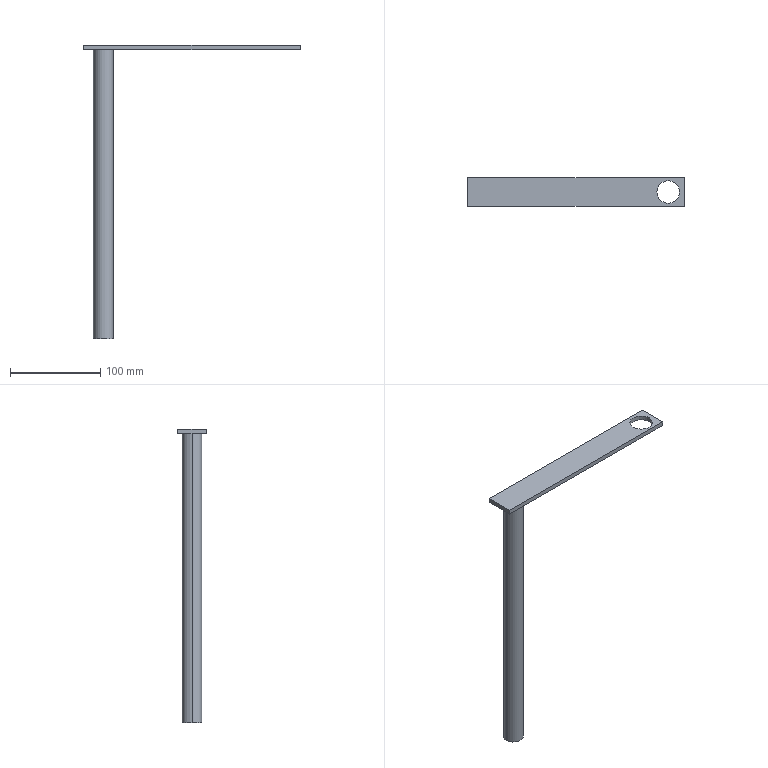Part | STEP file | 1 solid | 11 faces | box 240 x 32 x 325 mm | volume 157588 mm3 | plane 7 | cylinder 4 | commonest cylinder face diameters 22 x2 25 x2
STEP:
#1=CARTESIAN_POINT('',(0.,0.,0.));
#2=DIRECTION('',(0.,0.,1.));
#3=DIRECTION('',(1.,0.,0.));
#4=AXIS2_PLACEMENT_3D('',#1,#2,#3);
#5=CARTESIAN_POINT('',(-109.,0.,0.));
#6=VERTEX_POINT('',#5);
#7=CARTESIAN_POINT('',(-87.,0.,0.));
#8=VERTEX_POINT('',#7);
#9=CARTESIAN_POINT('',(-98.,0.,0.));
#10=DIRECTION('',(0.,0.,-1.));
#11=DIRECTION('',(-1.,0.,0.));
#12=AXIS2_PLACEMENT_3D('',#9,#10,#11);
#13=CIRCLE('',#12,11.);
#14=CARTESIAN_POINT('',(-98.,0.,-320.));
#15=DIRECTION('',(0.,0.,-1.));
#16=DIRECTION('',(-1.,0.,0.));
#17=AXIS2_PLACEMENT_3D('',#14,#15,#16);
#18=CYLINDRICAL_SURFACE('',#17,11.);
#19=CARTESIAN_POINT('',(0.,-320.));
#20=DIRECTION('',(1.,0.));
#21=VECTOR('',#20,1.);
#22=LINE('',#19,#21);
#23=(GEOMETRIC_REPRESENTATION_CONTEXT(2)PARAMETRIC_REPRESENTATION_CONTEXT()REPRESENTATION_CONTEXT('',''));
#24=DEFINITIONAL_REPRESENTATION('',(#22),#23);
#25=PCURVE('',#18,#24);
#26=CARTESIAN_POINT('',(0.,0.,0.));
#27=DIRECTION('',(0.,0.,1.));
#28=DIRECTION('',(1.,0.,0.));
#29=AXIS2_PLACEMENT_3D('',#26,#27,#28);
#30=PLANE('',#29);
#31=CARTESIAN_POINT('',(-109.,0.));
#32=CARTESIAN_POINT('',(-109.,19.053));
#33=CARTESIAN_POINT('',(-92.5,9.526));
#34=CARTESIAN_POINT('',(-76.,0.));
#35=CARTESIAN_POINT('',(-92.5,-9.526));
#36=CARTESIAN_POINT('',(-109.,-19.053));
#37=CARTESIAN_POINT('',(-109.,0.));
#38=(BOUNDED_CURVE()B_SPLINE_CURVE(2,(#31,#32,#33,#34,#35,#36,#37),.UNSPECIFIED.,.T.,.F.)B_SPLINE_CURVE_WITH_KNOTS((1,2,2,2,2,1),(-2.094,0.,2.094,4.189,6.283,8.378),.UNSPECIFIED.)CURVE()GEOMETRIC_REPRESENTATION_ITEM()RATIONAL_B_SPLINE_CURVE((1.,0.5,1.,0.5,1.,0.5,1.))REPRESENTATION_ITEM(''));
#39=(GEOMETRIC_REPRESENTATION_CONTEXT(2)PARAMETRIC_REPRESENTATION_CONTEXT()REPRESENTATION_CONTEXT('',''));
#40=DEFINITIONAL_REPRESENTATION('',(#38),#39);
#41=PCURVE('',#30,#40);
#42=SURFACE_CURVE('',#13,(#25,#41),.PCURVE_S1.);
#43=EDGE_CURVE('',#6,#8,#42,.T.);
#44=ORIENTED_EDGE('',*,*,#43,.T.);
#45=CARTESIAN_POINT('',(-87.,0.,-320.));
#46=VERTEX_POINT('',#45);
#47=CARTESIAN_POINT('',(-87.,0.,-320.));
#48=DIRECTION('',(0.,0.,-1.));
#49=VECTOR('',#48,1.);
#50=LINE('',#47,#49);
#51=CARTESIAN_POINT('',(3.142,0.));
#52=DIRECTION('',(0.,1.));
#53=VECTOR('',#52,1.);
#54=LINE('',#51,#53);
#55=(GEOMETRIC_REPRESENTATION_CONTEXT(2)PARAMETRIC_REPRESENTATION_CONTEXT()REPRESENTATION_CONTEXT('',''));
#56=DEFINITIONAL_REPRESENTATION('',(#54),#55);
#57=PCURVE('',#18,#56);
#58=CARTESIAN_POINT('',(-98.,0.,-320.));
#59=DIRECTION('',(0.,0.,-1.));
#60=DIRECTION('',(-1.,0.,0.));
#61=AXIS2_PLACEMENT_3D('',#58,#59,#60);
#62=CYLINDRICAL_SURFACE('',#61,11.);
#63=CARTESIAN_POINT('',(3.142,0.));
#64=DIRECTION('',(0.,1.));
#65=VECTOR('',#64,1.);
#66=LINE('',#63,#65);
#67=(GEOMETRIC_REPRESENTATION_CONTEXT(2)PARAMETRIC_REPRESENTATION_CONTEXT()REPRESENTATION_CONTEXT('',''));
#68=DEFINITIONAL_REPRESENTATION('',(#66),#67);
#69=PCURVE('',#62,#68);
#70=SURFACE_CURVE('',#50,(#57,#69),.PCURVE_S1.);
#71=EDGE_CURVE('',#8,#46,#70,.T.);
#72=ORIENTED_EDGE('',*,*,#71,.T.);
#73=CARTESIAN_POINT('',(-109.,0.,-320.));
#74=VERTEX_POINT('',#73);
#75=CARTESIAN_POINT('',(-98.,0.,-320.));
#76=DIRECTION('',(0.,0.,1.));
#77=DIRECTION('',(-1.,0.,0.));
#78=AXIS2_PLACEMENT_3D('',#75,#76,#77);
#79=CIRCLE('',#78,11.);
#80=CARTESIAN_POINT('',(6.283,0.));
#81=DIRECTION('',(-1.,0.));
#82=VECTOR('',#81,1.);
#83=LINE('',#80,#82);
#84=(GEOMETRIC_REPRESENTATION_CONTEXT(2)PARAMETRIC_REPRESENTATION_CONTEXT()REPRESENTATION_CONTEXT('',''));
#85=DEFINITIONAL_REPRESENTATION('',(#83),#84);
#86=PCURVE('',#18,#85);
#87=CARTESIAN_POINT('',(-98.,0.,-320.));
#88=DIRECTION('',(0.,0.,-1.));
#89=DIRECTION('',(-1.,0.,0.));
#90=AXIS2_PLACEMENT_3D('',#87,#88,#89);
#91=PLANE('',#90);
#92=CARTESIAN_POINT('',(11.,0.));
#93=CARTESIAN_POINT('',(11.,-19.053));
#94=CARTESIAN_POINT('',(-5.5,-9.526));
#95=CARTESIAN_POINT('',(-22.,0.));
#96=CARTESIAN_POINT('',(-5.5,9.526));
#97=CARTESIAN_POINT('',(11.,19.053));
#98=CARTESIAN_POINT('',(11.,0.));
#99=(BOUNDED_CURVE()B_SPLINE_CURVE(2,(#92,#93,#94,#95,#96,#97,#98),.UNSPECIFIED.,.T.,.F.)B_SPLINE_CURVE_WITH_KNOTS((1,2,2,2,2,1),(-2.094,0.,2.094,4.189,6.283,8.378),.UNSPECIFIED.)CURVE()GEOMETRIC_REPRESENTATION_ITEM()RATIONAL_B_SPLINE_CURVE((1.,0.5,1.,0.5,1.,0.5,1.))REPRESENTATION_ITEM(''));
#100=(GEOMETRIC_REPRESENTATION_CONTEXT(2)PARAMETRIC_REPRESENTATION_CONTEXT()REPRESENTATION_CONTEXT('',''));
#101=DEFINITIONAL_REPRESENTATION('',(#99),#100);
#102=PCURVE('',#91,#101);
#103=SURFACE_CURVE('',#79,(#86,#102),.PCURVE_S1.);
#104=EDGE_CURVE('',#46,#74,#103,.T.);
#105=ORIENTED_EDGE('',*,*,#104,.T.);
#106=CARTESIAN_POINT('',(-109.,0.,-320.));
#107=DIRECTION('',(0.,0.,-1.));
#108=VECTOR('',#107,1.);
#109=LINE('',#106,#108);
#110=CARTESIAN_POINT('',(0.,0.));
#111=DIRECTION('',(0.,1.));
#112=VECTOR('',#111,1.);
#113=LINE('',#110,#112);
#114=(GEOMETRIC_REPRESENTATION_CONTEXT(2)PARAMETRIC_REPRESENTATION_CONTEXT()REPRESENTATION_CONTEXT('',''));
#115=DEFINITIONAL_REPRESENTATION('',(#113),#114);
#116=PCURVE('',#18,#115);
#117=CARTESIAN_POINT('',(6.283,0.));
#118=DIRECTION('',(0.,1.));
#119=VECTOR('',#118,1.);
#120=LINE('',#117,#119);
#121=(GEOMETRIC_REPRESENTATION_CONTEXT(2)PARAMETRIC_REPRESENTATION_CONTEXT()REPRESENTATION_CONTEXT('',''));
#122=DEFINITIONAL_REPRESENTATION('',(#120),#121);
#123=PCURVE('',#62,#122);
#124=SURFACE_CURVE('',#109,(#116,#123),.PCURVE_S1.);
#125=EDGE_CURVE('',#6,#74,#124,.T.);
#126=ORIENTED_EDGE('',*,*,#125,.F.);
#127=EDGE_LOOP('',(#44,#72,#105,#126));
#128=FACE_BOUND('',#127,.T.);
#129=ADVANCED_FACE('',(#128),#18,.T.);
#130=CARTESIAN_POINT('',(89.5,0.,5.));
#131=VERTEX_POINT('',#130);
#132=CARTESIAN_POINT('',(89.5,0.,0.));
#133=VERTEX_POINT('',#132);
#134=CARTESIAN_POINT('',(89.5,0.,-18.));
#135=DIRECTION('',(0.,0.,-1.));
#136=VECTOR('',#135,1.);
#137=LINE('',#134,#136);
#138=CARTESIAN_POINT('',(102.,0.,-18.));
#139=DIRECTION('',(0.,0.,-1.));
#140=DIRECTION('',(-1.,0.,0.));
#141=AXIS2_PLACEMENT_3D('',#138,#139,#140);
#142=CYLINDRICAL_SURFACE('',#141,12.5);
#143=CARTESIAN_POINT('',(6.283,0.));
#144=DIRECTION('',(0.,1.));
#145=VECTOR('',#144,1.);
#146=LINE('',#143,#145);
#147=(GEOMETRIC_REPRESENTATION_CONTEXT(2)PARAMETRIC_REPRESENTATION_CONTEXT()REPRESENTATION_CONTEXT('',''));
#148=DEFINITIONAL_REPRESENTATION('',(#146),#147);
#149=PCURVE('',#142,#148);
#150=CARTESIAN_POINT('',(102.,0.,-18.));
#151=DIRECTION('',(0.,0.,-1.));
#152=DIRECTION('',(-1.,0.,0.));
#153=AXIS2_PLACEMENT_3D('',#150,#151,#152);
#154=CYLINDRICAL_SURFACE('',#153,12.5);
#155=CARTESIAN_POINT('',(0.,0.));
#156=DIRECTION('',(0.,1.));
#157=VECTOR('',#156,1.);
#158=LINE('',#155,#157);
#159=(GEOMETRIC_REPRESENTATION_CONTEXT(2)PARAMETRIC_REPRESENTATION_CONTEXT()REPRESENTATION_CONTEXT('',''));
#160=DEFINITIONAL_REPRESENTATION('',(#158),#159);
#161=PCURVE('',#154,#160);
#162=SURFACE_CURVE('',#137,(#149,#161),.PCURVE_S1.);
#163=EDGE_CURVE('',#131,#133,#162,.T.);
#164=ORIENTED_EDGE('',*,*,#163,.T.);
#165=CARTESIAN_POINT('',(114.5,0.,0.));
#166=VERTEX_POINT('',#165);
#167=CARTESIAN_POINT('',(102.,0.,0.));
#168=DIRECTION('',(0.,0.,-1.));
#169=DIRECTION('',(-1.,0.,0.));
#170=AXIS2_PLACEMENT_3D('',#167,#168,#169);
#171=CIRCLE('',#170,12.5);
#172=CARTESIAN_POINT('',(0.,-18.));
#173=DIRECTION('',(1.,0.));
#174=VECTOR('',#173,1.);
#175=LINE('',#172,#174);
#176=(GEOMETRIC_REPRESENTATION_CONTEXT(2)PARAMETRIC_REPRESENTATION_CONTEXT()REPRESENTATION_CONTEXT('',''));
#177=DEFINITIONAL_REPRESENTATION('',(#175),#176);
#178=PCURVE('',#142,#177);
#179=CARTESIAN_POINT('',(89.5,0.));
#180=CARTESIAN_POINT('',(89.5,21.651));
#181=CARTESIAN_POINT('',(108.25,10.825));
#182=CARTESIAN_POINT('',(127.,0.));
#183=CARTESIAN_POINT('',(108.25,-10.825));
#184=CARTESIAN_POINT('',(89.5,-21.651));
#185=CARTESIAN_POINT('',(89.5,0.));
#186=(BOUNDED_CURVE()B_SPLINE_CURVE(2,(#179,#180,#181,#182,#183,#184,#185),.UNSPECIFIED.,.T.,.F.)B_SPLINE_CURVE_WITH_KNOTS((1,2,2,2,2,1),(-2.094,0.,2.094,4.189,6.283,8.378),.UNSPECIFIED.)CURVE()GEOMETRIC_REPRESENTATION_ITEM()RATIONAL_B_SPLINE_CURVE((1.,0.5,1.,0.5,1.,0.5,1.))REPRESENTATION_ITEM(''));
#187=(GEOMETRIC_REPRESENTATION_CONTEXT(2)PARAMETRIC_REPRESENTATION_CONTEXT()REPRESENTATION_CONTEXT('',''));
#188=DEFINITIONAL_REPRESENTATION('',(#186),#187);
#189=PCURVE('',#30,#188);
#190=SURFACE_CURVE('',#171,(#178,#189),.PCURVE_S1.);
#191=EDGE_CURVE('',#166,#133,#190,.T.);
#192=ORIENTED_EDGE('',*,*,#191,.F.);
#193=CARTESIAN_POINT('',(114.5,0.,5.));
#194=VERTEX_POINT('',#193);
#195=CARTESIAN_POINT('',(114.5,0.,-18.));
#196=DIRECTION('',(0.,0.,-1.));
#197=VECTOR('',#196,1.);
#198=LINE('',#195,#197);
#199=CARTESIAN_POINT('',(3.142,0.));
#200=DIRECTION('',(0.,1.));
#201=VECTOR('',#200,1.);
#202=LINE('',#199,#201);
#203=(GEOMETRIC_REPRESENTATION_CONTEXT(2)PARAMETRIC_REPRESENTATION_CONTEXT()REPRESENTATION_CONTEXT('',''));
#204=DEFINITIONAL_REPRESENTATION('',(#202),#203);
#205=PCURVE('',#142,#204);
#206=CARTESIAN_POINT('',(3.142,0.));
#207=DIRECTION('',(0.,1.));
#208=VECTOR('',#207,1.);
#209=LINE('',#206,#208);
#210=(GEOMETRIC_REPRESENTATION_CONTEXT(2)PARAMETRIC_REPRESENTATION_CONTEXT()REPRESENTATION_CONTEXT('',''));
#211=DEFINITIONAL_REPRESENTATION('',(#209),#210);
#212=PCURVE('',#154,#211);
#213=SURFACE_CURVE('',#198,(#205,#212),.PCURVE_S1.);
#214=EDGE_CURVE('',#194,#166,#213,.T.);
#215=ORIENTED_EDGE('',*,*,#214,.F.);
#216=CARTESIAN_POINT('',(102.,0.,5.));
#217=DIRECTION('',(0.,0.,-1.));
#218=DIRECTION('',(-1.,0.,0.));
#219=AXIS2_PLACEMENT_3D('',#216,#217,#218);
#220=CIRCLE('',#219,12.5);
#221=CARTESIAN_POINT('',(0.,-23.));
#222=DIRECTION('',(1.,0.));
#223=VECTOR('',#222,1.);
#224=LINE('',#221,#223);
#225=(GEOMETRIC_REPRESENTATION_CONTEXT(2)PARAMETRIC_REPRESENTATION_CONTEXT()REPRESENTATION_CONTEXT('',''));
#226=DEFINITIONAL_REPRESENTATION('',(#224),#225);
#227=PCURVE('',#142,#226);
#228=CARTESIAN_POINT('',(0.,0.,5.));
#229=DIRECTION('',(0.,0.,1.));
#230=DIRECTION('',(1.,0.,0.));
#231=AXIS2_PLACEMENT_3D('',#228,#229,#230);
#232=PLANE('',#231);
#233=CARTESIAN_POINT('',(89.5,0.));
#234=CARTESIAN_POINT('',(89.5,21.651));
#235=CARTESIAN_POINT('',(108.25,10.825));
#236=CARTESIAN_POINT('',(127.,0.));
#237=CARTESIAN_POINT('',(108.25,-10.825));
#238=CARTESIAN_POINT('',(89.5,-21.651));
#239=CARTESIAN_POINT('',(89.5,0.));
#240=(BOUNDED_CURVE()B_SPLINE_CURVE(2,(#233,#234,#235,#236,#237,#238,#239),.UNSPECIFIED.,.T.,.F.)B_SPLINE_CURVE_WITH_KNOTS((1,2,2,2,2,1),(-2.094,0.,2.094,4.189,6.283,8.378),.UNSPECIFIED.)CURVE()GEOMETRIC_REPRESENTATION_ITEM()RATIONAL_B_SPLINE_CURVE((1.,0.5,1.,0.5,1.,0.5,1.))REPRESENTATION_ITEM(''));
#241=(GEOMETRIC_REPRESENTATION_CONTEXT(2)PARAMETRIC_REPRESENTATION_CONTEXT()REPRESENTATION_CONTEXT('',''));
#242=DEFINITIONAL_REPRESENTATION('',(#240),#241);
#243=PCURVE('',#232,#242);
#244=SURFACE_CURVE('',#220,(#227,#243),.PCURVE_S1.);
#245=EDGE_CURVE('',#194,#131,#244,.T.);
#246=ORIENTED_EDGE('',*,*,#245,.T.);
#247=EDGE_LOOP('',(#164,#192,#215,#246));
#248=FACE_BOUND('',#247,.F.);
#249=ADVANCED_FACE('',(#248),#142,.F.);
#250=ORIENTED_EDGE('',*,*,#71,.F.);
#251=CARTESIAN_POINT('',(-98.,0.,0.));
#252=DIRECTION('',(0.,0.,-1.));
#253=DIRECTION('',(-1.,0.,0.));
#254=AXIS2_PLACEMENT_3D('',#251,#252,#253);
#255=CIRCLE('',#254,11.);
#256=CARTESIAN_POINT('',(0.,-320.));
#257=DIRECTION('',(1.,0.));
#258=VECTOR('',#257,1.);
#259=LINE('',#256,#258);
#260=(GEOMETRIC_REPRESENTATION_CONTEXT(2)PARAMETRIC_REPRESENTATION_CONTEXT()REPRESENTATION_CONTEXT('',''));
#261=DEFINITIONAL_REPRESENTATION('',(#259),#260);
#262=PCURVE('',#62,#261);
#263=CARTESIAN_POINT('',(-109.,0.));
#264=CARTESIAN_POINT('',(-109.,19.053));
#265=CARTESIAN_POINT('',(-92.5,9.526));
#266=CARTESIAN_POINT('',(-76.,0.));
#267=CARTESIAN_POINT('',(-92.5,-9.526));
#268=CARTESIAN_POINT('',(-109.,-19.053));
#269=CARTESIAN_POINT('',(-109.,0.));
#270=(BOUNDED_CURVE()B_SPLINE_CURVE(2,(#263,#264,#265,#266,#267,#268,#269),.UNSPECIFIED.,.T.,.F.)B_SPLINE_CURVE_WITH_KNOTS((1,2,2,2,2,1),(-2.094,0.,2.094,4.189,6.283,8.378),.UNSPECIFIED.)CURVE()GEOMETRIC_REPRESENTATION_ITEM()RATIONAL_B_SPLINE_CURVE((1.,0.5,1.,0.5,1.,0.5,1.))REPRESENTATION_ITEM(''));
#271=(GEOMETRIC_REPRESENTATION_CONTEXT(2)PARAMETRIC_REPRESENTATION_CONTEXT()REPRESENTATION_CONTEXT('',''));
#272=DEFINITIONAL_REPRESENTATION('',(#270),#271);
#273=PCURVE('',#30,#272);
#274=SURFACE_CURVE('',#255,(#262,#273),.PCURVE_S1.);
#275=EDGE_CURVE('',#8,#6,#274,.T.);
#276=ORIENTED_EDGE('',*,*,#275,.T.);
#277=ORIENTED_EDGE('',*,*,#125,.T.);
#278=CARTESIAN_POINT('',(-98.,0.,-320.));
#279=DIRECTION('',(0.,0.,1.));
#280=DIRECTION('',(-1.,0.,0.));
#281=AXIS2_PLACEMENT_3D('',#278,#279,#280);
#282=CIRCLE('',#281,11.);
#283=CARTESIAN_POINT('',(6.283,0.));
#284=DIRECTION('',(-1.,0.));
#285=VECTOR('',#284,1.);
#286=LINE('',#283,#285);
#287=(GEOMETRIC_REPRESENTATION_CONTEXT(2)PARAMETRIC_REPRESENTATION_CONTEXT()REPRESENTATION_CONTEXT('',''));
#288=DEFINITIONAL_REPRESENTATION('',(#286),#287);
#289=PCURVE('',#62,#288);
#290=CARTESIAN_POINT('',(11.,0.));
#291=CARTESIAN_POINT('',(11.,-19.053));
#292=CARTESIAN_POINT('',(-5.5,-9.526));
#293=CARTESIAN_POINT('',(-22.,0.));
#294=CARTESIAN_POINT('',(-5.5,9.526));
#295=CARTESIAN_POINT('',(11.,19.053));
#296=CARTESIAN_POINT('',(11.,0.));
#297=(BOUNDED_CURVE()B_SPLINE_CURVE(2,(#290,#291,#292,#293,#294,#295,#296),.UNSPECIFIED.,.T.,.F.)B_SPLINE_CURVE_WITH_KNOTS((1,2,2,2,2,1),(-2.094,0.,2.094,4.189,6.283,8.378),.UNSPECIFIED.)CURVE()GEOMETRIC_REPRESENTATION_ITEM()RATIONAL_B_SPLINE_CURVE((1.,0.5,1.,0.5,1.,0.5,1.))REPRESENTATION_ITEM(''));
#298=(GEOMETRIC_REPRESENTATION_CONTEXT(2)PARAMETRIC_REPRESENTATION_CONTEXT()REPRESENTATION_CONTEXT('',''));
#299=DEFINITIONAL_REPRESENTATION('',(#297),#298);
#300=PCURVE('',#91,#299);
#301=SURFACE_CURVE('',#282,(#289,#300),.PCURVE_S1.);
#302=EDGE_CURVE('',#74,#46,#301,.T.);
#303=ORIENTED_EDGE('',*,*,#302,.T.);
#304=EDGE_LOOP('',(#250,#276,#277,#303));
#305=FACE_BOUND('',#304,.T.);
#306=ADVANCED_FACE('',(#305),#62,.T.);
#307=CARTESIAN_POINT('',(102.,0.,0.));
#308=DIRECTION('',(0.,0.,-1.));
#309=DIRECTION('',(-1.,0.,0.));
#310=AXIS2_PLACEMENT_3D('',#307,#308,#309);
#311=CIRCLE('',#310,12.5);
#312=CARTESIAN_POINT('',(89.5,0.));
#313=CARTESIAN_POINT('',(89.5,21.651));
#314=CARTESIAN_POINT('',(108.25,10.825));
#315=CARTESIAN_POINT('',(127.,0.));
#316=CARTESIAN_POINT('',(108.25,-10.825));
#317=CARTESIAN_POINT('',(89.5,-21.651));
#318=CARTESIAN_POINT('',(89.5,0.));
#319=(BOUNDED_CURVE()B_SPLINE_CURVE(2,(#312,#313,#314,#315,#316,#317,#318),.UNSPECIFIED.,.T.,.F.)B_SPLINE_CURVE_WITH_KNOTS((1,2,2,2,2,1),(-2.094,0.,2.094,4.189,6.283,8.378),.UNSPECIFIED.)CURVE()GEOMETRIC_REPRESENTATION_ITEM()RATIONAL_B_SPLINE_CURVE((1.,0.5,1.,0.5,1.,0.5,1.))REPRESENTATION_ITEM(''));
#320=(GEOMETRIC_REPRESENTATION_CONTEXT(2)PARAMETRIC_REPRESENTATION_CONTEXT()REPRESENTATION_CONTEXT('',''));
#321=DEFINITIONAL_REPRESENTATION('',(#319),#320);
#322=PCURVE('',#30,#321);
#323=CARTESIAN_POINT('',(0.,-18.));
#324=DIRECTION('',(1.,0.));
#325=VECTOR('',#324,1.);
#326=LINE('',#323,#325);
#327=(GEOMETRIC_REPRESENTATION_CONTEXT(2)PARAMETRIC_REPRESENTATION_CONTEXT()REPRESENTATION_CONTEXT('',''));
#328=DEFINITIONAL_REPRESENTATION('',(#326),#327);
#329=PCURVE('',#154,#328);
#330=SURFACE_CURVE('',#311,(#322,#329),.PCURVE_S1.);
#331=EDGE_CURVE('',#133,#166,#330,.T.);
#332=ORIENTED_EDGE('',*,*,#331,.F.);
#333=ORIENTED_EDGE('',*,*,#191,.F.);
#334=EDGE_LOOP('',(#332,#333));
#335=FACE_BOUND('',#334,.T.);
#336=ORIENTED_EDGE('',*,*,#43,.F.);
#337=ORIENTED_EDGE('',*,*,#275,.F.);
#338=EDGE_LOOP('',(#336,#337));
#339=FACE_BOUND('',#338,.T.);
#340=CARTESIAN_POINT('',(-120.,-16.,0.));
#341=VERTEX_POINT('',#340);
#342=CARTESIAN_POINT('',(120.,-16.,0.));
#343=VERTEX_POINT('',#342);
#344=CARTESIAN_POINT('',(0.,-16.,0.));
#345=DIRECTION('',(1.,0.,0.));
#346=VECTOR('',#345,1.);
#347=LINE('',#344,#346);
#348=CARTESIAN_POINT('',(0.,-16.));
#349=DIRECTION('',(1.,0.));
#350=VECTOR('',#349,1.);
#351=LINE('',#348,#350);
#352=(GEOMETRIC_REPRESENTATION_CONTEXT(2)PARAMETRIC_REPRESENTATION_CONTEXT()REPRESENTATION_CONTEXT('',''));
#353=DEFINITIONAL_REPRESENTATION('',(#351),#352);
#354=PCURVE('',#30,#353);
#355=CARTESIAN_POINT('',(-120.,-16.,5.));
#356=DIRECTION('',(0.,1.,0.));
#357=DIRECTION('',(0.,0.,1.));
#358=AXIS2_PLACEMENT_3D('',#355,#356,#357);
#359=PLANE('',#358);
#360=CARTESIAN_POINT('',(-5.,120.));
#361=DIRECTION('',(0.,1.));
#362=VECTOR('',#361,1.);
#363=LINE('',#360,#362);
#364=(GEOMETRIC_REPRESENTATION_CONTEXT(2)PARAMETRIC_REPRESENTATION_CONTEXT()REPRESENTATION_CONTEXT('',''));
#365=DEFINITIONAL_REPRESENTATION('',(#363),#364);
#366=PCURVE('',#359,#365);
#367=SURFACE_CURVE('',#347,(#354,#366),.PCURVE_S1.);
#368=EDGE_CURVE('',#341,#343,#367,.T.);
#369=ORIENTED_EDGE('',*,*,#368,.F.);
#370=CARTESIAN_POINT('',(-120.,16.,0.));
#371=VERTEX_POINT('',#370);
#372=CARTESIAN_POINT('',(-120.,0.,0.));
#373=DIRECTION('',(0.,-1.,0.));
#374=VECTOR('',#373,1.);
#375=LINE('',#372,#374);
#376=CARTESIAN_POINT('',(-120.,0.));
#377=DIRECTION('',(0.,-1.));
#378=VECTOR('',#377,1.);
#379=LINE('',#376,#378);
#380=(GEOMETRIC_REPRESENTATION_CONTEXT(2)PARAMETRIC_REPRESENTATION_CONTEXT()REPRESENTATION_CONTEXT('',''));
#381=DEFINITIONAL_REPRESENTATION('',(#379),#380);
#382=PCURVE('',#30,#381);
#383=CARTESIAN_POINT('',(-120.,16.,5.));
#384=DIRECTION('',(1.,0.,0.));
#385=DIRECTION('',(0.,0.,-1.));
#386=AXIS2_PLACEMENT_3D('',#383,#384,#385);
#387=PLANE('',#386);
#388=CARTESIAN_POINT('',(5.,-16.));
#389=DIRECTION('',(0.,-1.));
#390=VECTOR('',#389,1.);
#391=LINE('',#388,#390);
#392=(GEOMETRIC_REPRESENTATION_CONTEXT(2)PARAMETRIC_REPRESENTATION_CONTEXT()REPRESENTATION_CONTEXT('',''));
#393=DEFINITIONAL_REPRESENTATION('',(#391),#392);
#394=PCURVE('',#387,#393);
#395=SURFACE_CURVE('',#375,(#382,#394),.PCURVE_S1.);
#396=EDGE_CURVE('',#371,#341,#395,.T.);
#397=ORIENTED_EDGE('',*,*,#396,.F.);
#398=CARTESIAN_POINT('',(120.,16.,0.));
#399=VERTEX_POINT('',#398);
#400=CARTESIAN_POINT('',(0.,16.,0.));
#401=DIRECTION('',(-1.,0.,0.));
#402=VECTOR('',#401,1.);
#403=LINE('',#400,#402);
#404=CARTESIAN_POINT('',(0.,16.));
#405=DIRECTION('',(-1.,0.));
#406=VECTOR('',#405,1.);
#407=LINE('',#404,#406);
#408=(GEOMETRIC_REPRESENTATION_CONTEXT(2)PARAMETRIC_REPRESENTATION_CONTEXT()REPRESENTATION_CONTEXT('',''));
#409=DEFINITIONAL_REPRESENTATION('',(#407),#408);
#410=PCURVE('',#30,#409);
#411=CARTESIAN_POINT('',(-120.,16.,5.));
#412=DIRECTION('',(0.,-1.,0.));
#413=DIRECTION('',(0.,0.,-1.));
#414=AXIS2_PLACEMENT_3D('',#411,#412,#413);
#415=PLANE('',#414);
#416=CARTESIAN_POINT('',(5.,120.));
#417=DIRECTION('',(0.,-1.));
#418=VECTOR('',#417,1.);
#419=LINE('',#416,#418);
#420=(GEOMETRIC_REPRESENTATION_CONTEXT(2)PARAMETRIC_REPRESENTATION_CONTEXT()REPRESENTATION_CONTEXT('',''));
#421=DEFINITIONAL_REPRESENTATION('',(#419),#420);
#422=PCURVE('',#415,#421);
#423=SURFACE_CURVE('',#403,(#410,#422),.PCURVE_S1.);
#424=EDGE_CURVE('',#399,#371,#423,.T.);
#425=ORIENTED_EDGE('',*,*,#424,.F.);
#426=CARTESIAN_POINT('',(120.,0.,0.));
#427=DIRECTION('',(0.,1.,0.));
#428=VECTOR('',#427,1.);
#429=LINE('',#426,#428);
#430=CARTESIAN_POINT('',(120.,0.));
#431=DIRECTION('',(0.,1.));
#432=VECTOR('',#431,1.);
#433=LINE('',#430,#432);
#434=(GEOMETRIC_REPRESENTATION_CONTEXT(2)PARAMETRIC_REPRESENTATION_CONTEXT()REPRESENTATION_CONTEXT('',''));
#435=DEFINITIONAL_REPRESENTATION('',(#433),#434);
#436=PCURVE('',#30,#435);
#437=CARTESIAN_POINT('',(120.,16.,5.));
#438=DIRECTION('',(-1.,0.,0.));
#439=DIRECTION('',(0.,0.,1.));
#440=AXIS2_PLACEMENT_3D('',#437,#438,#439);
#441=PLANE('',#440);
#442=CARTESIAN_POINT('',(-5.,-16.));
#443=DIRECTION('',(0.,1.));
#444=VECTOR('',#443,1.);
#445=LINE('',#442,#444);
#446=(GEOMETRIC_REPRESENTATION_CONTEXT(2)PARAMETRIC_REPRESENTATION_CONTEXT()REPRESENTATION_CONTEXT('',''));
#447=DEFINITIONAL_REPRESENTATION('',(#445),#446);
#448=PCURVE('',#441,#447);
#449=SURFACE_CURVE('',#429,(#436,#448),.PCURVE_S1.);
#450=EDGE_CURVE('',#343,#399,#449,.T.);
#451=ORIENTED_EDGE('',*,*,#450,.F.);
#452=EDGE_LOOP('',(#369,#397,#425,#451));
#453=FACE_BOUND('',#452,.T.);
#454=ADVANCED_FACE('',(#335,#339,#453),#30,.F.);
#455=ORIENTED_EDGE('',*,*,#302,.F.);
#456=ORIENTED_EDGE('',*,*,#104,.F.);
#457=EDGE_LOOP('',(#455,#456));
#458=FACE_BOUND('',#457,.T.);
#459=ADVANCED_FACE('',(#458),#91,.T.);
#460=ORIENTED_EDGE('',*,*,#331,.F.);
#461=ORIENTED_EDGE('',*,*,#163,.F.);
#462=CARTESIAN_POINT('',(102.,0.,5.));
#463=DIRECTION('',(0.,0.,-1.));
#464=DIRECTION('',(-1.,0.,0.));
#465=AXIS2_PLACEMENT_3D('',#462,#463,#464);
#466=CIRCLE('',#465,12.5);
#467=CARTESIAN_POINT('',(0.,-23.));
#468=DIRECTION('',(1.,0.));
#469=VECTOR('',#468,1.);
#470=LINE('',#467,#469);
#471=(GEOMETRIC_REPRESENTATION_CONTEXT(2)PARAMETRIC_REPRESENTATION_CONTEXT()REPRESENTATION_CONTEXT('',''));
#472=DEFINITIONAL_REPRESENTATION('',(#470),#471);
#473=PCURVE('',#154,#472);
#474=CARTESIAN_POINT('',(89.5,0.));
#475=CARTESIAN_POINT('',(89.5,21.651));
#476=CARTESIAN_POINT('',(108.25,10.825));
#477=CARTESIAN_POINT('',(127.,0.));
#478=CARTESIAN_POINT('',(108.25,-10.825));
#479=CARTESIAN_POINT('',(89.5,-21.651));
#480=CARTESIAN_POINT('',(89.5,0.));
#481=(BOUNDED_CURVE()B_SPLINE_CURVE(2,(#474,#475,#476,#477,#478,#479,#480),.UNSPECIFIED.,.T.,.F.)B_SPLINE_CURVE_WITH_KNOTS((1,2,2,2,2,1),(-2.094,0.,2.094,4.189,6.283,8.378),.UNSPECIFIED.)CURVE()GEOMETRIC_REPRESENTATION_ITEM()RATIONAL_B_SPLINE_CURVE((1.,0.5,1.,0.5,1.,0.5,1.))REPRESENTATION_ITEM(''));
#482=(GEOMETRIC_REPRESENTATION_CONTEXT(2)PARAMETRIC_REPRESENTATION_CONTEXT()REPRESENTATION_CONTEXT('',''));
#483=DEFINITIONAL_REPRESENTATION('',(#481),#482);
#484=PCURVE('',#232,#483);
#485=SURFACE_CURVE('',#466,(#473,#484),.PCURVE_S1.);
#486=EDGE_CURVE('',#131,#194,#485,.T.);
#487=ORIENTED_EDGE('',*,*,#486,.T.);
#488=ORIENTED_EDGE('',*,*,#214,.T.);
#489=EDGE_LOOP('',(#460,#461,#487,#488));
#490=FACE_BOUND('',#489,.F.);
#491=ADVANCED_FACE('',(#490),#154,.F.);
#492=CARTESIAN_POINT('',(120.,16.,5.));
#493=VERTEX_POINT('',#492);
#494=CARTESIAN_POINT('',(120.,16.,5.));
#495=DIRECTION('',(0.,0.,-1.));
#496=VECTOR('',#495,1.);
#497=LINE('',#494,#496);
#498=CARTESIAN_POINT('',(0.,0.));
#499=DIRECTION('',(-1.,0.));
#500=VECTOR('',#499,1.);
#501=LINE('',#498,#500);
#502=(GEOMETRIC_REPRESENTATION_CONTEXT(2)PARAMETRIC_REPRESENTATION_CONTEXT()REPRESENTATION_CONTEXT('',''));
#503=DEFINITIONAL_REPRESENTATION('',(#501),#502);
#504=PCURVE('',#441,#503);
#505=CARTESIAN_POINT('',(0.,240.));
#506=DIRECTION('',(1.,0.));
#507=VECTOR('',#506,1.);
#508=LINE('',#505,#507);
#509=(GEOMETRIC_REPRESENTATION_CONTEXT(2)PARAMETRIC_REPRESENTATION_CONTEXT()REPRESENTATION_CONTEXT('',''));
#510=DEFINITIONAL_REPRESENTATION('',(#508),#509);
#511=PCURVE('',#415,#510);
#512=SURFACE_CURVE('',#497,(#504,#511),.PCURVE_S1.);
#513=EDGE_CURVE('',#493,#399,#512,.T.);
#514=ORIENTED_EDGE('',*,*,#513,.F.);
#515=CARTESIAN_POINT('',(120.,-16.,5.));
#516=VERTEX_POINT('',#515);
#517=CARTESIAN_POINT('',(120.,16.,5.));
#518=DIRECTION('',(0.,1.,0.));
#519=VECTOR('',#518,1.);
#520=LINE('',#517,#519);
#521=CARTESIAN_POINT('',(0.,0.));
#522=DIRECTION('',(0.,1.));
#523=VECTOR('',#522,1.);
#524=LINE('',#521,#523);
#525=(GEOMETRIC_REPRESENTATION_CONTEXT(2)PARAMETRIC_REPRESENTATION_CONTEXT()REPRESENTATION_CONTEXT('',''));
#526=DEFINITIONAL_REPRESENTATION('',(#524),#525);
#527=PCURVE('',#441,#526);
#528=CARTESIAN_POINT('',(120.,16.));
#529=DIRECTION('',(0.,1.));
#530=VECTOR('',#529,1.);
#531=LINE('',#528,#530);
#532=(GEOMETRIC_REPRESENTATION_CONTEXT(2)PARAMETRIC_REPRESENTATION_CONTEXT()REPRESENTATION_CONTEXT('',''));
#533=DEFINITIONAL_REPRESENTATION('',(#531),#532);
#534=PCURVE('',#232,#533);
#535=SURFACE_CURVE('',#520,(#527,#534),.PCURVE_S1.);
#536=EDGE_CURVE('',#516,#493,#535,.T.);
#537=ORIENTED_EDGE('',*,*,#536,.F.);
#538=CARTESIAN_POINT('',(120.,-16.,5.));
#539=DIRECTION('',(0.,0.,1.));
#540=VECTOR('',#539,1.);
#541=LINE('',#538,#540);
#542=CARTESIAN_POINT('',(0.,-32.));
#543=DIRECTION('',(1.,0.));
#544=VECTOR('',#543,1.);
#545=LINE('',#542,#544);
#546=(GEOMETRIC_REPRESENTATION_CONTEXT(2)PARAMETRIC_REPRESENTATION_CONTEXT()REPRESENTATION_CONTEXT('',''));
#547=DEFINITIONAL_REPRESENTATION('',(#545),#546);
#548=PCURVE('',#441,#547);
#549=CARTESIAN_POINT('',(0.,240.));
#550=DIRECTION('',(1.,0.));
#551=VECTOR('',#550,1.);
#552=LINE('',#549,#551);
#553=(GEOMETRIC_REPRESENTATION_CONTEXT(2)PARAMETRIC_REPRESENTATION_CONTEXT()REPRESENTATION_CONTEXT('',''));
#554=DEFINITIONAL_REPRESENTATION('',(#552),#553);
#555=PCURVE('',#359,#554);
#556=SURFACE_CURVE('',#541,(#548,#555),.PCURVE_S1.);
#557=EDGE_CURVE('',#343,#516,#556,.T.);
#558=ORIENTED_EDGE('',*,*,#557,.F.);
#559=ORIENTED_EDGE('',*,*,#450,.T.);
#560=EDGE_LOOP('',(#514,#537,#558,#559));
#561=FACE_BOUND('',#560,.T.);
#562=ADVANCED_FACE('',(#561),#441,.F.);
#563=ORIENTED_EDGE('',*,*,#557,.T.);
#564=CARTESIAN_POINT('',(-120.,-16.,5.));
#565=VERTEX_POINT('',#564);
#566=CARTESIAN_POINT('',(-120.,-16.,5.));
#567=DIRECTION('',(1.,0.,0.));
#568=VECTOR('',#567,1.);
#569=LINE('',#566,#568);
#570=CARTESIAN_POINT('',(0.,0.));
#571=DIRECTION('',(0.,1.));
#572=VECTOR('',#571,1.);
#573=LINE('',#570,#572);
#574=(GEOMETRIC_REPRESENTATION_CONTEXT(2)PARAMETRIC_REPRESENTATION_CONTEXT()REPRESENTATION_CONTEXT('',''));
#575=DEFINITIONAL_REPRESENTATION('',(#573),#574);
#576=PCURVE('',#359,#575);
#577=CARTESIAN_POINT('',(-120.,-16.));
#578=DIRECTION('',(1.,0.));
#579=VECTOR('',#578,1.);
#580=LINE('',#577,#579);
#581=(GEOMETRIC_REPRESENTATION_CONTEXT(2)PARAMETRIC_REPRESENTATION_CONTEXT()REPRESENTATION_CONTEXT('',''));
#582=DEFINITIONAL_REPRESENTATION('',(#580),#581);
#583=PCURVE('',#232,#582);
#584=SURFACE_CURVE('',#569,(#576,#583),.PCURVE_S1.);
#585=EDGE_CURVE('',#565,#516,#584,.T.);
#586=ORIENTED_EDGE('',*,*,#585,.F.);
#587=CARTESIAN_POINT('',(-120.,-16.,5.));
#588=DIRECTION('',(0.,0.,1.));
#589=VECTOR('',#588,1.);
#590=LINE('',#587,#589);
#591=CARTESIAN_POINT('',(0.,0.));
#592=DIRECTION('',(1.,0.));
#593=VECTOR('',#592,1.);
#594=LINE('',#591,#593);
#595=(GEOMETRIC_REPRESENTATION_CONTEXT(2)PARAMETRIC_REPRESENTATION_CONTEXT()REPRESENTATION_CONTEXT('',''));
#596=DEFINITIONAL_REPRESENTATION('',(#594),#595);
#597=PCURVE('',#359,#596);
#598=CARTESIAN_POINT('',(0.,-32.));
#599=DIRECTION('',(-1.,0.));
#600=VECTOR('',#599,1.);
#601=LINE('',#598,#600);
#602=(GEOMETRIC_REPRESENTATION_CONTEXT(2)PARAMETRIC_REPRESENTATION_CONTEXT()REPRESENTATION_CONTEXT('',''));
#603=DEFINITIONAL_REPRESENTATION('',(#601),#602);
#604=PCURVE('',#387,#603);
#605=SURFACE_CURVE('',#590,(#597,#604),.PCURVE_S1.);
#606=EDGE_CURVE('',#341,#565,#605,.T.);
#607=ORIENTED_EDGE('',*,*,#606,.F.);
#608=ORIENTED_EDGE('',*,*,#368,.T.);
#609=EDGE_LOOP('',(#563,#586,#607,#608));
#610=FACE_BOUND('',#609,.T.);
#611=ADVANCED_FACE('',(#610),#359,.F.);
#612=ORIENTED_EDGE('',*,*,#606,.T.);
#613=CARTESIAN_POINT('',(-120.,16.,5.));
#614=VERTEX_POINT('',#613);
#615=CARTESIAN_POINT('',(-120.,16.,5.));
#616=DIRECTION('',(0.,-1.,0.));
#617=VECTOR('',#616,1.);
#618=LINE('',#615,#617);
#619=CARTESIAN_POINT('',(0.,0.));
#620=DIRECTION('',(0.,-1.));
#621=VECTOR('',#620,1.);
#622=LINE('',#619,#621);
#623=(GEOMETRIC_REPRESENTATION_CONTEXT(2)PARAMETRIC_REPRESENTATION_CONTEXT()REPRESENTATION_CONTEXT('',''));
#624=DEFINITIONAL_REPRESENTATION('',(#622),#623);
#625=PCURVE('',#387,#624);
#626=CARTESIAN_POINT('',(-120.,16.));
#627=DIRECTION('',(0.,-1.));
#628=VECTOR('',#627,1.);
#629=LINE('',#626,#628);
#630=(GEOMETRIC_REPRESENTATION_CONTEXT(2)PARAMETRIC_REPRESENTATION_CONTEXT()REPRESENTATION_CONTEXT('',''));
#631=DEFINITIONAL_REPRESENTATION('',(#629),#630);
#632=PCURVE('',#232,#631);
#633=SURFACE_CURVE('',#618,(#625,#632),.PCURVE_S1.);
#634=EDGE_CURVE('',#614,#565,#633,.T.);
#635=ORIENTED_EDGE('',*,*,#634,.F.);
#636=CARTESIAN_POINT('',(-120.,16.,5.));
#637=DIRECTION('',(0.,0.,1.));
#638=VECTOR('',#637,1.);
#639=LINE('',#636,#638);
#640=CARTESIAN_POINT('',(0.,0.));
#641=DIRECTION('',(-1.,0.));
#642=VECTOR('',#641,1.);
#643=LINE('',#640,#642);
#644=(GEOMETRIC_REPRESENTATION_CONTEXT(2)PARAMETRIC_REPRESENTATION_CONTEXT()REPRESENTATION_CONTEXT('',''));
#645=DEFINITIONAL_REPRESENTATION('',(#643),#644);
#646=PCURVE('',#387,#645);
#647=CARTESIAN_POINT('',(0.,0.));
#648=DIRECTION('',(-1.,0.));
#649=VECTOR('',#648,1.);
#650=LINE('',#647,#649);
#651=(GEOMETRIC_REPRESENTATION_CONTEXT(2)PARAMETRIC_REPRESENTATION_CONTEXT()REPRESENTATION_CONTEXT('',''));
#652=DEFINITIONAL_REPRESENTATION('',(#650),#651);
#653=PCURVE('',#415,#652);
#654=SURFACE_CURVE('',#639,(#646,#653),.PCURVE_S1.);
#655=EDGE_CURVE('',#371,#614,#654,.T.);
#656=ORIENTED_EDGE('',*,*,#655,.F.);
#657=ORIENTED_EDGE('',*,*,#396,.T.);
#658=EDGE_LOOP('',(#612,#635,#656,#657));
#659=FACE_BOUND('',#658,.T.);
#660=ADVANCED_FACE('',(#659),#387,.F.);
#661=ORIENTED_EDGE('',*,*,#655,.T.);
#662=CARTESIAN_POINT('',(-120.,16.,5.));
#663=DIRECTION('',(-1.,0.,0.));
#664=VECTOR('',#663,1.);
#665=LINE('',#662,#664);
#666=CARTESIAN_POINT('',(0.,0.));
#667=DIRECTION('',(0.,-1.));
#668=VECTOR('',#667,1.);
#669=LINE('',#666,#668);
#670=(GEOMETRIC_REPRESENTATION_CONTEXT(2)PARAMETRIC_REPRESENTATION_CONTEXT()REPRESENTATION_CONTEXT('',''));
#671=DEFINITIONAL_REPRESENTATION('',(#669),#670);
#672=PCURVE('',#415,#671);
#673=CARTESIAN_POINT('',(-120.,16.));
#674=DIRECTION('',(-1.,0.));
#675=VECTOR('',#674,1.);
#676=LINE('',#673,#675);
#677=(GEOMETRIC_REPRESENTATION_CONTEXT(2)PARAMETRIC_REPRESENTATION_CONTEXT()REPRESENTATION_CONTEXT('',''));
#678=DEFINITIONAL_REPRESENTATION('',(#676),#677);
#679=PCURVE('',#232,#678);
#680=SURFACE_CURVE('',#665,(#672,#679),.PCURVE_S1.);
#681=EDGE_CURVE('',#493,#614,#680,.T.);
#682=ORIENTED_EDGE('',*,*,#681,.F.);
#683=ORIENTED_EDGE('',*,*,#513,.T.);
#684=ORIENTED_EDGE('',*,*,#424,.T.);
#685=EDGE_LOOP('',(#661,#682,#683,#684));
#686=FACE_BOUND('',#685,.T.);
#687=ADVANCED_FACE('',(#686),#415,.F.);
#688=ORIENTED_EDGE('',*,*,#486,.T.);
#689=ORIENTED_EDGE('',*,*,#245,.T.);
#690=EDGE_LOOP('',(#688,#689));
#691=FACE_BOUND('',#690,.T.);
#692=ORIENTED_EDGE('',*,*,#634,.T.);
#693=ORIENTED_EDGE('',*,*,#585,.T.);
#694=ORIENTED_EDGE('',*,*,#536,.T.);
#695=ORIENTED_EDGE('',*,*,#681,.T.);
#696=EDGE_LOOP('',(#692,#693,#694,#695));
#697=FACE_BOUND('',#696,.T.);
#698=ADVANCED_FACE('',(#691,#697),#232,.T.);
#699=CLOSED_SHELL('',(#129,#249,#306,#454,#459,#491,#562,#611,#660,#687,#698));
#700=MANIFOLD_SOLID_BREP('',#699);
#701=(LENGTH_UNIT()NAMED_UNIT(*)SI_UNIT(.MILLI.,.METRE.));
#702=UNCERTAINTY_MEASURE_WITH_UNIT(LENGTH_MEASURE(0.0000001),#701,'','');
#703=(NAMED_UNIT(*)PLANE_ANGLE_UNIT()SI_UNIT($,.RADIAN.));
#704=(NAMED_UNIT(*)SI_UNIT($,.STERADIAN.)SOLID_ANGLE_UNIT());
#705=(GEOMETRIC_REPRESENTATION_CONTEXT(3)GLOBAL_UNCERTAINTY_ASSIGNED_CONTEXT((#702))GLOBAL_UNIT_ASSIGNED_CONTEXT((#701,#703,#704))REPRESENTATION_CONTEXT('',''));
#706=ADVANCED_BREP_SHAPE_REPRESENTATION('',(#4,#700),#705);